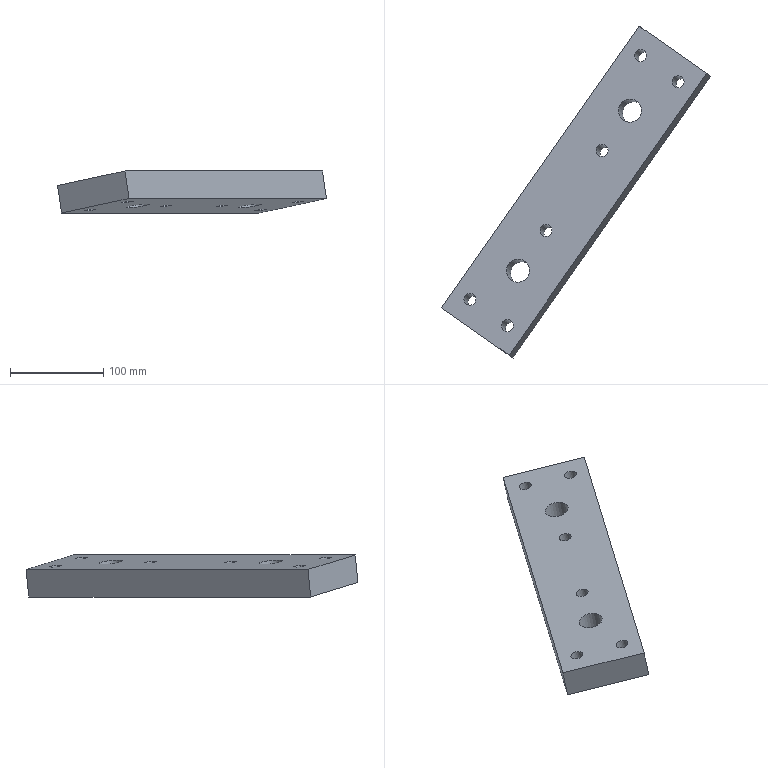Part | NX | features solid 2 | 1 solid | 14 faces | box 289.094 x 356.912 x 45.173 mm | volume 945656 mm3 | cylinder 8 | plane 6 | commonest cylinder face diameters 13 x6 25 x2
STEP:
#1=CARTESIAN_POINT('',(-256.799,245.356,-127.697));
#2=VERTEX_POINT('',#1);
#3=CARTESIAN_POINT('',(-263.232,245.356,-128.627));
#4=DIRECTION('',(-0.1422,0.0996,0.9848));
#5=DIRECTION('',(0.9897,0.,0.143));
#6=AXIS2_PLACEMENT_3D('',#3,#4,#5);
#7=CIRCLE('',#6,6.5);
#8=EDGE_CURVE('',#2,#2,#7,.F.);
#9=ORIENTED_EDGE('',*,*,#8,.F.);
#10=EDGE_LOOP('',(#9));
#11=FACE_BOUND('',#10,.T.);
#12=CARTESIAN_POINT('',(-113.59,535.728,-136.38));
#13=VERTEX_POINT('',#12);
#14=CARTESIAN_POINT('',(-120.023,535.728,-137.309));
#15=DIRECTION('',(-0.1422,0.0996,0.9848));
#16=DIRECTION('',(0.9897,0.,0.143));
#17=AXIS2_PLACEMENT_3D('',#14,#15,#16);
#18=CIRCLE('',#17,6.5);
#19=EDGE_CURVE('',#13,#13,#18,.T.);
#20=ORIENTED_EDGE('',*,*,#19,.T.);
#21=EDGE_LOOP('',(#20));
#22=FACE_BOUND('',#21,.T.);
#23=CARTESIAN_POINT('',(-73.254,507.484,-127.697));
#24=VERTEX_POINT('',#23);
#25=CARTESIAN_POINT('',(-79.688,507.484,-128.627));
#26=DIRECTION('',(-0.1422,0.0996,0.9848));
#27=DIRECTION('',(0.9897,0.,0.143));
#28=AXIS2_PLACEMENT_3D('',#25,#26,#27);
#29=CIRCLE('',#28,6.5);
#30=EDGE_CURVE('',#24,#24,#29,.F.);
#31=ORIENTED_EDGE('',*,*,#30,.F.);
#32=EDGE_LOOP('',(#31));
#33=FACE_BOUND('',#32,.T.);
#34=CARTESIAN_POINT('',(-334.041,264.417,-140.782));
#35=VERTEX_POINT('',#34);
#36=CARTESIAN_POINT('',(-121.818,567.504,-140.782));
#37=VERTEX_POINT('',#36);
#38=CARTESIAN_POINT('',(-259.476,370.907,-140.782));
#39=DIRECTION('',(-0.5736,-0.8192,0.));
#40=VECTOR('',#39,1000.);
#41=LINE('',#38,#40);
#42=EDGE_CURVE('',#35,#37,#41,.F.);
#43=ORIENTED_EDGE('',*,*,#42,.T.);
#44=CARTESIAN_POINT('',(-49.214,516.666,-125.154));
#45=VERTEX_POINT('',#44);
#46=CARTESIAN_POINT('',(-49.12,516.6,-125.133));
#47=DIRECTION('',(-0.8067,0.5649,-0.1736));
#48=VECTOR('',#47,1000.);
#49=LINE('',#46,#48);
#50=EDGE_CURVE('',#45,#37,#49,.T.);
#51=ORIENTED_EDGE('',*,*,#50,.F.);
#52=CARTESIAN_POINT('',(-261.437,213.58,-125.154));
#53=VERTEX_POINT('',#52);
#54=CARTESIAN_POINT('',(-186.872,320.069,-125.154));
#55=DIRECTION('',(-0.5736,-0.8192,0.));
#56=VECTOR('',#55,1000.);
#57=LINE('',#54,#56);
#58=EDGE_CURVE('',#53,#45,#57,.F.);
#59=ORIENTED_EDGE('',*,*,#58,.F.);
#60=CARTESIAN_POINT('',(-261.343,213.514,-125.133));
#61=DIRECTION('',(-0.8067,0.5649,-0.1736));
#62=VECTOR('',#61,1000.);
#63=LINE('',#60,#62);
#64=EDGE_CURVE('',#53,#35,#63,.T.);
#65=ORIENTED_EDGE('',*,*,#64,.T.);
#66=EDGE_LOOP('',(#43,#51,#59,#65));
#67=FACE_BOUND('',#66,.T.);
#68=CARTESIAN_POINT('',(-247.622,292.905,-131.181));
#69=VERTEX_POINT('',#68);
#70=CARTESIAN_POINT('',(-251.853,304.531,-132.968));
#71=DIRECTION('',(-0.1422,0.0996,0.9848));
#72=DIRECTION('',(0.3385,-0.93,0.143));
#73=AXIS2_PLACEMENT_3D('',#70,#71,#72);
#74=CIRCLE('',#73,12.5);
#75=EDGE_CURVE('',#69,#69,#74,.F.);
#76=ORIENTED_EDGE('',*,*,#75,.F.);
#77=EDGE_LOOP('',(#76));
#78=FACE_BOUND('',#77,.T.);
#79=CARTESIAN_POINT('',(-127.171,464.927,-131.181));
#80=VERTEX_POINT('',#79);
#81=CARTESIAN_POINT('',(-131.402,476.553,-132.968));
#82=DIRECTION('',(-0.1422,0.0996,0.9848));
#83=DIRECTION('',(0.3385,-0.93,0.143));
#84=AXIS2_PLACEMENT_3D('',#81,#82,#83);
#85=CIRCLE('',#84,12.5);
#86=EDGE_CURVE('',#80,#80,#85,.T.);
#87=ORIENTED_EDGE('',*,*,#86,.T.);
#88=EDGE_LOOP('',(#87));
#89=FACE_BOUND('',#88,.T.);
#90=CARTESIAN_POINT('',(-155.081,433.547,-132.039));
#91=VERTEX_POINT('',#90);
#92=CARTESIAN_POINT('',(-161.515,433.547,-132.968));
#93=DIRECTION('',(-0.1422,0.0996,0.9848));
#94=DIRECTION('',(0.9897,0.,0.143));
#95=AXIS2_PLACEMENT_3D('',#92,#93,#94);
#96=CIRCLE('',#95,6.5);
#97=EDGE_CURVE('',#91,#91,#96,.F.);
#98=ORIENTED_EDGE('',*,*,#97,.F.);
#99=EDGE_LOOP('',(#98));
#100=FACE_BOUND('',#99,.T.);
#101=CARTESIAN_POINT('',(-215.307,347.536,-132.039));
#102=VERTEX_POINT('',#101);
#103=CARTESIAN_POINT('',(-221.74,347.536,-132.968));
#104=DIRECTION('',(-0.1422,0.0996,0.9848));
#105=DIRECTION('',(0.9897,0.,0.143));
#106=AXIS2_PLACEMENT_3D('',#103,#104,#105);
#107=CIRCLE('',#106,6.5);
#108=EDGE_CURVE('',#102,#102,#107,.F.);
#109=ORIENTED_EDGE('',*,*,#108,.F.);
#110=EDGE_LOOP('',(#109));
#111=FACE_BOUND('',#110,.T.);
#112=CARTESIAN_POINT('',(-297.134,273.599,-136.38));
#113=VERTEX_POINT('',#112);
#114=CARTESIAN_POINT('',(-303.567,273.599,-137.309));
#115=DIRECTION('',(-0.1422,0.0996,0.9848));
#116=DIRECTION('',(0.9897,0.,0.143));
#117=AXIS2_PLACEMENT_3D('',#114,#115,#116);
#118=CIRCLE('',#117,6.5);
#119=EDGE_CURVE('',#113,#113,#118,.T.);
#120=ORIENTED_EDGE('',*,*,#119,.T.);
#121=EDGE_LOOP('',(#120));
#122=FACE_BOUND('',#121,.T.);
#123=CARTESIAN_POINT('',(-186.778,320.003,-125.133));
#124=DIRECTION('',(-0.1422,0.0996,0.9848));
#125=DIRECTION('',(-0.8067,0.5649,-0.1736));
#126=AXIS2_PLACEMENT_3D('',#123,#124,#125);
#127=PLANE('',#126);
#128=ADVANCED_FACE('',(#11,#22,#33,#67,#78,#89,#100,#111,#122),#127,.F.);
#129=CARTESIAN_POINT('',(-261.066,248.344,-98.153));
#130=VERTEX_POINT('',#129);
#131=CARTESIAN_POINT('',(-267.499,248.344,-99.082));
#132=DIRECTION('',(-0.1422,0.0996,0.9848));
#133=DIRECTION('',(0.9897,0.,0.143));
#134=AXIS2_PLACEMENT_3D('',#131,#132,#133);
#135=CIRCLE('',#134,6.5);
#136=EDGE_CURVE('',#130,#130,#135,.F.);
#137=ORIENTED_EDGE('',*,*,#136,.T.);
#138=EDGE_LOOP('',(#137));
#139=FACE_BOUND('',#138,.T.);
#140=CARTESIAN_POINT('',(-117.857,538.716,-106.836));
#141=VERTEX_POINT('',#140);
#142=CARTESIAN_POINT('',(-124.29,538.716,-107.765));
#143=DIRECTION('',(-0.1422,0.0996,0.9848));
#144=DIRECTION('',(0.9897,0.,0.143));
#145=AXIS2_PLACEMENT_3D('',#142,#143,#144);
#146=CIRCLE('',#145,6.5);
#147=EDGE_CURVE('',#141,#141,#146,.T.);
#148=ORIENTED_EDGE('',*,*,#147,.F.);
#149=EDGE_LOOP('',(#148));
#150=FACE_BOUND('',#149,.T.);
#151=CARTESIAN_POINT('',(-77.522,510.472,-98.153));
#152=VERTEX_POINT('',#151);
#153=CARTESIAN_POINT('',(-83.955,510.472,-99.082));
#154=DIRECTION('',(-0.1422,0.0996,0.9848));
#155=DIRECTION('',(0.9897,0.,0.143));
#156=AXIS2_PLACEMENT_3D('',#153,#154,#155);
#157=CIRCLE('',#156,6.5);
#158=EDGE_CURVE('',#152,#152,#157,.F.);
#159=ORIENTED_EDGE('',*,*,#158,.T.);
#160=EDGE_LOOP('',(#159));
#161=FACE_BOUND('',#160,.T.);
#162=CARTESIAN_POINT('',(-265.705,216.568,-95.609));
#163=VERTEX_POINT('',#162);
#164=CARTESIAN_POINT('',(-338.308,267.405,-111.238));
#165=VERTEX_POINT('',#164);
#166=CARTESIAN_POINT('',(-265.61,216.502,-95.589));
#167=DIRECTION('',(-0.8067,0.5649,-0.1736));
#168=VECTOR('',#167,1000.);
#169=LINE('',#166,#168);
#170=EDGE_CURVE('',#163,#165,#169,.T.);
#171=ORIENTED_EDGE('',*,*,#170,.F.);
#172=CARTESIAN_POINT('',(-53.481,519.654,-95.609));
#173=VERTEX_POINT('',#172);
#174=CARTESIAN_POINT('',(-179.668,339.441,-95.609));
#175=DIRECTION('',(-0.5736,-0.8192,0.));
#176=VECTOR('',#175,1000.);
#177=LINE('',#174,#176);
#178=EDGE_CURVE('',#163,#173,#177,.F.);
#179=ORIENTED_EDGE('',*,*,#178,.T.);
#180=CARTESIAN_POINT('',(-126.085,570.492,-111.238));
#181=VERTEX_POINT('',#180);
#182=CARTESIAN_POINT('',(-53.387,519.588,-95.589));
#183=DIRECTION('',(-0.8067,0.5649,-0.1736));
#184=VECTOR('',#183,1000.);
#185=LINE('',#182,#184);
#186=EDGE_CURVE('',#173,#181,#185,.T.);
#187=ORIENTED_EDGE('',*,*,#186,.T.);
#188=CARTESIAN_POINT('',(-252.272,390.278,-111.238));
#189=DIRECTION('',(-0.5736,-0.8192,0.));
#190=VECTOR('',#189,1000.);
#191=LINE('',#188,#190);
#192=EDGE_CURVE('',#165,#181,#191,.F.);
#193=ORIENTED_EDGE('',*,*,#192,.F.);
#194=EDGE_LOOP('',(#171,#179,#187,#193));
#195=FACE_BOUND('',#194,.T.);
#196=CARTESIAN_POINT('',(-251.889,295.893,-101.637));
#197=VERTEX_POINT('',#196);
#198=CARTESIAN_POINT('',(-256.12,307.519,-103.424));
#199=DIRECTION('',(-0.1422,0.0996,0.9848));
#200=DIRECTION('',(0.3385,-0.93,0.143));
#201=AXIS2_PLACEMENT_3D('',#198,#199,#200);
#202=CIRCLE('',#201,12.5);
#203=EDGE_CURVE('',#197,#197,#202,.F.);
#204=ORIENTED_EDGE('',*,*,#203,.T.);
#205=EDGE_LOOP('',(#204));
#206=FACE_BOUND('',#205,.T.);
#207=CARTESIAN_POINT('',(-131.438,467.915,-101.637));
#208=VERTEX_POINT('',#207);
#209=CARTESIAN_POINT('',(-135.669,479.541,-103.424));
#210=DIRECTION('',(-0.1422,0.0996,0.9848));
#211=DIRECTION('',(0.3385,-0.93,0.143));
#212=AXIS2_PLACEMENT_3D('',#209,#210,#211);
#213=CIRCLE('',#212,12.5);
#214=EDGE_CURVE('',#208,#208,#213,.T.);
#215=ORIENTED_EDGE('',*,*,#214,.F.);
#216=EDGE_LOOP('',(#215));
#217=FACE_BOUND('',#216,.T.);
#218=CARTESIAN_POINT('',(-159.349,436.535,-102.494));
#219=VERTEX_POINT('',#218);
#220=CARTESIAN_POINT('',(-165.782,436.535,-103.424));
#221=DIRECTION('',(-0.1422,0.0996,0.9848));
#222=DIRECTION('',(0.9897,0.,0.143));
#223=AXIS2_PLACEMENT_3D('',#220,#221,#222);
#224=CIRCLE('',#223,6.5);
#225=EDGE_CURVE('',#219,#219,#224,.F.);
#226=ORIENTED_EDGE('',*,*,#225,.T.);
#227=EDGE_LOOP('',(#226));
#228=FACE_BOUND('',#227,.T.);
#229=CARTESIAN_POINT('',(-219.574,350.524,-102.494));
#230=VERTEX_POINT('',#229);
#231=CARTESIAN_POINT('',(-226.008,350.524,-103.424));
#232=DIRECTION('',(-0.1422,0.0996,0.9848));
#233=DIRECTION('',(0.9897,0.,0.143));
#234=AXIS2_PLACEMENT_3D('',#231,#232,#233);
#235=CIRCLE('',#234,6.5);
#236=EDGE_CURVE('',#230,#230,#235,.F.);
#237=ORIENTED_EDGE('',*,*,#236,.T.);
#238=EDGE_LOOP('',(#237));
#239=FACE_BOUND('',#238,.T.);
#240=CARTESIAN_POINT('',(-301.401,276.587,-106.836));
#241=VERTEX_POINT('',#240);
#242=CARTESIAN_POINT('',(-307.835,276.587,-107.765));
#243=DIRECTION('',(-0.1422,0.0996,0.9848));
#244=DIRECTION('',(0.9897,0.,0.143));
#245=AXIS2_PLACEMENT_3D('',#242,#243,#244);
#246=CIRCLE('',#245,6.5);
#247=EDGE_CURVE('',#241,#241,#246,.T.);
#248=ORIENTED_EDGE('',*,*,#247,.F.);
#249=EDGE_LOOP('',(#248));
#250=FACE_BOUND('',#249,.T.);
#251=CARTESIAN_POINT('',(-191.045,322.991,-95.589));
#252=DIRECTION('',(-0.1422,0.0996,0.9848));
#253=DIRECTION('',(-0.8067,0.5649,-0.1736));
#254=AXIS2_PLACEMENT_3D('',#251,#252,#253);
#255=PLANE('',#254);
#256=ADVANCED_FACE('',(#139,#150,#161,#195,#206,#217,#228,#239,#250),#255,.T.);
#257=CARTESIAN_POINT('',(-336.886,266.409,-121.086));
#258=DIRECTION('',(-0.1422,0.0996,0.9848));
#259=VECTOR('',#258,1000.);
#260=LINE('',#257,#259);
#261=EDGE_CURVE('',#165,#35,#260,.F.);
#262=ORIENTED_EDGE('',*,*,#261,.F.);
#263=ORIENTED_EDGE('',*,*,#192,.T.);
#264=CARTESIAN_POINT('',(-120.395,566.508,-150.63));
#265=DIRECTION('',(-0.1422,0.0996,0.9848));
#266=VECTOR('',#265,1000.);
#267=LINE('',#264,#266);
#268=EDGE_CURVE('',#181,#37,#267,.F.);
#269=ORIENTED_EDGE('',*,*,#268,.T.);
#270=ORIENTED_EDGE('',*,*,#42,.F.);
#271=EDGE_LOOP('',(#262,#263,#269,#270));
#272=FACE_BOUND('',#271,.T.);
#273=CARTESIAN_POINT('',(-250.849,389.282,-121.086));
#274=DIRECTION('',(0.8067,-0.5649,0.1736));
#275=DIRECTION('',(0.2171,0.01006,-0.9761));
#276=AXIS2_PLACEMENT_3D('',#273,#274,#275);
#277=PLANE('',#276);
#278=ADVANCED_FACE('',(#272),#277,.F.);
#279=ORIENTED_EDGE('',*,*,#261,.T.);
#280=ORIENTED_EDGE('',*,*,#64,.F.);
#281=CARTESIAN_POINT('',(-264.282,215.572,-105.457));
#282=DIRECTION('',(-0.1422,0.0996,0.9848));
#283=VECTOR('',#282,1000.);
#284=LINE('',#281,#283);
#285=EDGE_CURVE('',#163,#53,#284,.F.);
#286=ORIENTED_EDGE('',*,*,#285,.F.);
#287=ORIENTED_EDGE('',*,*,#170,.T.);
#288=EDGE_LOOP('',(#279,#280,#286,#287));
#289=FACE_BOUND('',#288,.T.);
#290=CARTESIAN_POINT('',(-259.92,212.518,-134.981));
#291=DIRECTION('',(0.5736,0.8192,0.));
#292=DIRECTION('',(0.7698,-0.539,-0.342));
#293=AXIS2_PLACEMENT_3D('',#290,#291,#292);
#294=PLANE('',#293);
#295=ADVANCED_FACE('',(#289),#294,.F.);
#296=ORIENTED_EDGE('',*,*,#58,.T.);
#297=CARTESIAN_POINT('',(-47.792,515.67,-135.002));
#298=DIRECTION('',(-0.1422,0.0996,0.9848));
#299=VECTOR('',#298,1000.);
#300=LINE('',#297,#299);
#301=EDGE_CURVE('',#173,#45,#300,.F.);
#302=ORIENTED_EDGE('',*,*,#301,.F.);
#303=ORIENTED_EDGE('',*,*,#178,.F.);
#304=ORIENTED_EDGE('',*,*,#285,.T.);
#305=EDGE_LOOP('',(#296,#302,#303,#304));
#306=FACE_BOUND('',#305,.T.);
#307=CARTESIAN_POINT('',(-178.246,338.445,-105.457));
#308=DIRECTION('',(0.8067,-0.5649,0.1736));
#309=DIRECTION('',(0.2171,0.01006,-0.9761));
#310=AXIS2_PLACEMENT_3D('',#307,#308,#309);
#311=PLANE('',#310);
#312=ADVANCED_FACE('',(#306),#311,.T.);
#313=ORIENTED_EDGE('',*,*,#75,.T.);
#314=EDGE_LOOP('',(#313));
#315=FACE_BOUND('',#314,.T.);
#316=ORIENTED_EDGE('',*,*,#203,.F.);
#317=EDGE_LOOP('',(#316));
#318=FACE_BOUND('',#317,.T.);
#319=CARTESIAN_POINT('',(-249.719,303.037,-147.74));
#320=DIRECTION('',(0.1422,-0.0996,-0.9848));
#321=DIRECTION('',(0.3452,0.9374,-0.04494));
#322=AXIS2_PLACEMENT_3D('',#319,#320,#321);
#323=CYLINDRICAL_SURFACE('',#322,12.5);
#324=ADVANCED_FACE('',(#315,#318),#323,.F.);
#325=ORIENTED_EDGE('',*,*,#268,.F.);
#326=ORIENTED_EDGE('',*,*,#186,.F.);
#327=ORIENTED_EDGE('',*,*,#301,.T.);
#328=ORIENTED_EDGE('',*,*,#50,.T.);
#329=EDGE_LOOP('',(#325,#326,#327,#328));
#330=FACE_BOUND('',#329,.T.);
#331=CARTESIAN_POINT('',(-47.697,515.604,-134.981));
#332=DIRECTION('',(-0.5736,-0.8192,0.));
#333=DIRECTION('',(0.7698,-0.539,-0.342));
#334=AXIS2_PLACEMENT_3D('',#331,#332,#333);
#335=PLANE('',#334);
#336=ADVANCED_FACE('',(#330),#335,.F.);
#337=ORIENTED_EDGE('',*,*,#86,.F.);
#338=EDGE_LOOP('',(#337));
#339=FACE_BOUND('',#338,.T.);
#340=ORIENTED_EDGE('',*,*,#214,.T.);
#341=EDGE_LOOP('',(#340));
#342=FACE_BOUND('',#341,.T.);
#343=CARTESIAN_POINT('',(-129.268,475.059,-147.74));
#344=DIRECTION('',(0.1422,-0.0996,-0.9848));
#345=DIRECTION('',(-0.7628,-0.645,-0.04494));
#346=AXIS2_PLACEMENT_3D('',#343,#344,#345);
#347=CYLINDRICAL_SURFACE('',#346,12.5);
#348=ADVANCED_FACE('',(#339,#342),#347,.F.);
#349=ORIENTED_EDGE('',*,*,#30,.T.);
#350=EDGE_LOOP('',(#349));
#351=FACE_BOUND('',#350,.T.);
#352=ORIENTED_EDGE('',*,*,#158,.F.);
#353=EDGE_LOOP('',(#352));
#354=FACE_BOUND('',#353,.T.);
#355=CARTESIAN_POINT('',(-69.73,500.512,-197.563));
#356=DIRECTION('',(-0.1422,0.0996,0.9848));
#357=DIRECTION('',(0.9897,0.,0.143));
#358=AXIS2_PLACEMENT_3D('',#355,#356,#357);
#359=CYLINDRICAL_SURFACE('',#358,6.5);
#360=ADVANCED_FACE('',(#351,#354),#359,.F.);
#361=ORIENTED_EDGE('',*,*,#19,.F.);
#362=EDGE_LOOP('',(#361));
#363=FACE_BOUND('',#362,.T.);
#364=ORIENTED_EDGE('',*,*,#147,.T.);
#365=EDGE_LOOP('',(#364));
#366=FACE_BOUND('',#365,.T.);
#367=CARTESIAN_POINT('',(-110.066,528.756,-206.246));
#368=DIRECTION('',(-0.1422,0.0996,0.9848));
#369=DIRECTION('',(0.9897,0.,0.143));
#370=AXIS2_PLACEMENT_3D('',#367,#368,#369);
#371=CYLINDRICAL_SURFACE('',#370,6.5);
#372=ADVANCED_FACE('',(#363,#366),#371,.F.);
#373=ORIENTED_EDGE('',*,*,#97,.T.);
#374=EDGE_LOOP('',(#373));
#375=FACE_BOUND('',#374,.T.);
#376=ORIENTED_EDGE('',*,*,#225,.F.);
#377=EDGE_LOOP('',(#376));
#378=FACE_BOUND('',#377,.T.);
#379=CARTESIAN_POINT('',(-151.558,426.575,-201.904));
#380=DIRECTION('',(-0.1422,0.0996,0.9848));
#381=DIRECTION('',(0.9897,0.,0.143));
#382=AXIS2_PLACEMENT_3D('',#379,#380,#381);
#383=CYLINDRICAL_SURFACE('',#382,6.5);
#384=ADVANCED_FACE('',(#375,#378),#383,.F.);
#385=ORIENTED_EDGE('',*,*,#108,.T.);
#386=EDGE_LOOP('',(#385));
#387=FACE_BOUND('',#386,.T.);
#388=ORIENTED_EDGE('',*,*,#236,.F.);
#389=EDGE_LOOP('',(#388));
#390=FACE_BOUND('',#389,.T.);
#391=CARTESIAN_POINT('',(-211.783,340.564,-201.904));
#392=DIRECTION('',(-0.1422,0.0996,0.9848));
#393=DIRECTION('',(0.9897,0.,0.143));
#394=AXIS2_PLACEMENT_3D('',#391,#392,#393);
#395=CYLINDRICAL_SURFACE('',#394,6.5);
#396=ADVANCED_FACE('',(#387,#390),#395,.F.);
#397=ORIENTED_EDGE('',*,*,#119,.F.);
#398=EDGE_LOOP('',(#397));
#399=FACE_BOUND('',#398,.T.);
#400=ORIENTED_EDGE('',*,*,#247,.T.);
#401=EDGE_LOOP('',(#400));
#402=FACE_BOUND('',#401,.T.);
#403=CARTESIAN_POINT('',(-293.61,266.627,-206.246));
#404=DIRECTION('',(-0.1422,0.0996,0.9848));
#405=DIRECTION('',(0.9897,0.,0.143));
#406=AXIS2_PLACEMENT_3D('',#403,#404,#405);
#407=CYLINDRICAL_SURFACE('',#406,6.5);
#408=ADVANCED_FACE('',(#399,#402),#407,.F.);
#409=ORIENTED_EDGE('',*,*,#8,.T.);
#410=EDGE_LOOP('',(#409));
#411=FACE_BOUND('',#410,.T.);
#412=ORIENTED_EDGE('',*,*,#136,.F.);
#413=EDGE_LOOP('',(#412));
#414=FACE_BOUND('',#413,.T.);
#415=CARTESIAN_POINT('',(-253.275,238.384,-197.563));
#416=DIRECTION('',(-0.1422,0.0996,0.9848));
#417=DIRECTION('',(0.9897,0.,0.143));
#418=AXIS2_PLACEMENT_3D('',#415,#416,#417);
#419=CYLINDRICAL_SURFACE('',#418,6.5);
#420=ADVANCED_FACE('',(#411,#414),#419,.F.);
#421=CLOSED_SHELL('',(#128,#256,#278,#295,#312,#324,#336,#348,#360,#372,#384,#396,#408,#420));
#422=MANIFOLD_SOLID_BREP('',#421);
#423=(LENGTH_UNIT()NAMED_UNIT(*)SI_UNIT(.MILLI.,.METRE.));
#424=UNCERTAINTY_MEASURE_WITH_UNIT(LENGTH_MEASURE(0.00001),#423,'','');
#425=(NAMED_UNIT(*)PLANE_ANGLE_UNIT()SI_UNIT($,.RADIAN.));
#426=(NAMED_UNIT(*)SI_UNIT($,.STERADIAN.)SOLID_ANGLE_UNIT());
#427=(GEOMETRIC_REPRESENTATION_CONTEXT(3)GLOBAL_UNCERTAINTY_ASSIGNED_CONTEXT((#424))GLOBAL_UNIT_ASSIGNED_CONTEXT((#423,#425,#426))REPRESENTATION_CONTEXT('',''));
#428=ADVANCED_BREP_SHAPE_REPRESENTATION('',(#422),#427);